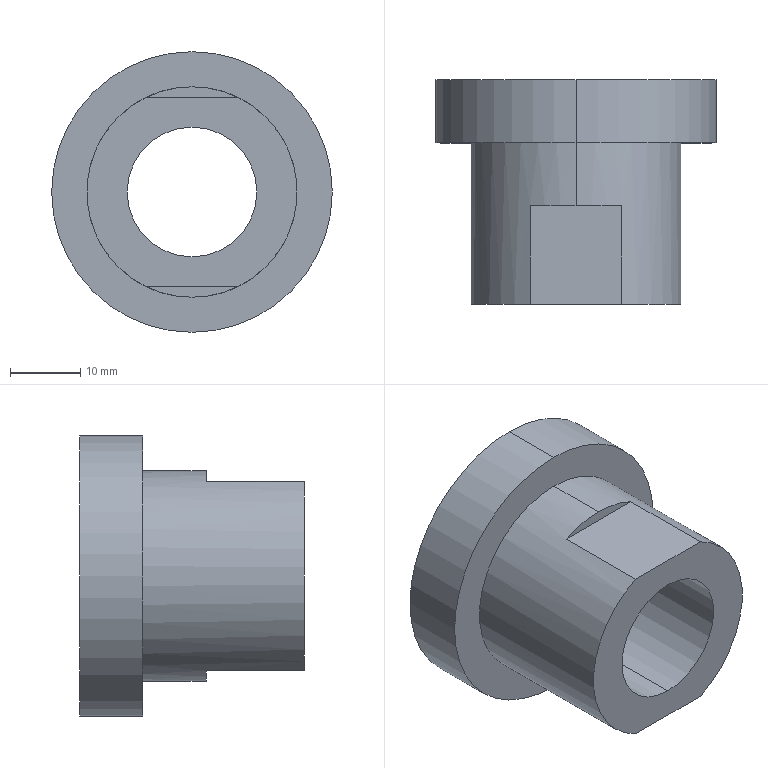Part | SolidWorks | features ICE 2, Extrusion 1, HoleWzd 1 | 1 solid | 13 faces | box 40 x 32 x 40 mm | volume 18596 mm3 | plane 7 | cylinder 6 | commonest cylinder face diameters 18.5 x2 30 x2 40 x2
STEP:
#1=CARTESIAN_POINT('',(0.,0.,-9.25));
#2=VERTEX_POINT('',#1);
#3=CARTESIAN_POINT('',(0.,0.,9.25));
#4=VERTEX_POINT('',#3);
#5=CARTESIAN_POINT('',(0.,0.,0.));
#6=DIRECTION('',(0.,1.,0.));
#7=DIRECTION('',(0.,0.,1.));
#8=AXIS2_PLACEMENT_3D('',#5,#6,#7);
#9=CIRCLE('',#8,9.25);
#10=EDGE_CURVE('',#2,#4,#9,.T.);
#11=ORIENTED_EDGE('',*,*,#10,.F.);
#12=CARTESIAN_POINT('',(0.,32.,-9.25));
#13=VERTEX_POINT('',#12);
#14=CARTESIAN_POINT('',(0.,32.,-9.25));
#15=DIRECTION('',(0.,1.,0.));
#16=VECTOR('',#15,1000.);
#17=LINE('',#14,#16);
#18=EDGE_CURVE('',#2,#13,#17,.T.);
#19=ORIENTED_EDGE('',*,*,#18,.T.);
#20=CARTESIAN_POINT('',(0.,32.,9.25));
#21=VERTEX_POINT('',#20);
#22=CARTESIAN_POINT('',(0.,32.,0.));
#23=DIRECTION('',(0.,1.,0.));
#24=DIRECTION('',(0.,0.,1.));
#25=AXIS2_PLACEMENT_3D('',#22,#23,#24);
#26=CIRCLE('',#25,9.25);
#27=EDGE_CURVE('',#13,#21,#26,.T.);
#28=ORIENTED_EDGE('',*,*,#27,.T.);
#29=CARTESIAN_POINT('',(0.,32.,9.25));
#30=DIRECTION('',(0.,1.,0.));
#31=VECTOR('',#30,1000.);
#32=LINE('',#29,#31);
#33=EDGE_CURVE('',#4,#21,#32,.T.);
#34=ORIENTED_EDGE('',*,*,#33,.F.);
#35=EDGE_LOOP('',(#11,#19,#28,#34));
#36=FACE_OUTER_BOUND('',#35,.T.);
#37=CARTESIAN_POINT('',(0.,32.,0.));
#38=DIRECTION('',(0.,1.,0.));
#39=DIRECTION('',(0.,0.,1.));
#40=AXIS2_PLACEMENT_3D('',#37,#38,#39);
#41=CYLINDRICAL_SURFACE('',#40,9.25);
#42=ADVANCED_FACE('',(#36),#41,.F.);
#43=CARTESIAN_POINT('',(0.,23.,-15.));
#44=VERTEX_POINT('',#43);
#45=CARTESIAN_POINT('',(0.,23.,15.));
#46=VERTEX_POINT('',#45);
#47=CARTESIAN_POINT('',(0.,23.,0.));
#48=DIRECTION('',(0.,-1.,0.));
#49=DIRECTION('',(0.,0.,-1.));
#50=AXIS2_PLACEMENT_3D('',#47,#48,#49);
#51=CIRCLE('',#50,15.);
#52=EDGE_CURVE('',#44,#46,#51,.T.);
#53=ORIENTED_EDGE('',*,*,#52,.T.);
#54=CARTESIAN_POINT('',(0.,14.,15.));
#55=VERTEX_POINT('',#54);
#56=CARTESIAN_POINT('',(0.,23.,15.));
#57=DIRECTION('',(0.,-1.,0.));
#58=VECTOR('',#57,1000.);
#59=LINE('',#56,#58);
#60=EDGE_CURVE('',#46,#55,#59,.T.);
#61=ORIENTED_EDGE('',*,*,#60,.T.);
#62=CARTESIAN_POINT('',(6.538,14.,13.5));
#63=VERTEX_POINT('',#62);
#64=CARTESIAN_POINT('',(0.,14.,0.));
#65=DIRECTION('',(0.,-1.,0.));
#66=DIRECTION('',(0.,0.,1.));
#67=AXIS2_PLACEMENT_3D('',#64,#65,#66);
#68=CIRCLE('',#67,15.);
#69=EDGE_CURVE('',#63,#55,#68,.T.);
#70=ORIENTED_EDGE('',*,*,#69,.F.);
#71=CARTESIAN_POINT('',(6.538,0.,13.5));
#72=VERTEX_POINT('',#71);
#73=CARTESIAN_POINT('',(6.538,23.,13.5));
#74=DIRECTION('',(0.,1.,0.));
#75=VECTOR('',#74,1000.);
#76=LINE('',#73,#75);
#77=EDGE_CURVE('',#72,#63,#76,.T.);
#78=ORIENTED_EDGE('',*,*,#77,.F.);
#79=CARTESIAN_POINT('',(6.538,0.,-13.5));
#80=VERTEX_POINT('',#79);
#81=CARTESIAN_POINT('',(0.,0.,0.));
#82=DIRECTION('',(0.,-1.,0.));
#83=DIRECTION('',(0.,0.,-1.));
#84=AXIS2_PLACEMENT_3D('',#81,#82,#83);
#85=CIRCLE('',#84,15.);
#86=EDGE_CURVE('',#80,#72,#85,.T.);
#87=ORIENTED_EDGE('',*,*,#86,.F.);
#88=CARTESIAN_POINT('',(6.538,14.,-13.5));
#89=VERTEX_POINT('',#88);
#90=CARTESIAN_POINT('',(6.538,23.,-13.5));
#91=DIRECTION('',(0.,-1.,0.));
#92=VECTOR('',#91,1000.);
#93=LINE('',#90,#92);
#94=EDGE_CURVE('',#89,#80,#93,.T.);
#95=ORIENTED_EDGE('',*,*,#94,.F.);
#96=CARTESIAN_POINT('',(0.,14.,-15.));
#97=VERTEX_POINT('',#96);
#98=CARTESIAN_POINT('',(0.,14.,0.));
#99=DIRECTION('',(0.,-1.,0.));
#100=DIRECTION('',(0.,0.,1.));
#101=AXIS2_PLACEMENT_3D('',#98,#99,#100);
#102=CIRCLE('',#101,15.);
#103=EDGE_CURVE('',#97,#89,#102,.T.);
#104=ORIENTED_EDGE('',*,*,#103,.F.);
#105=CARTESIAN_POINT('',(0.,23.,-15.));
#106=DIRECTION('',(0.,-1.,0.));
#107=VECTOR('',#106,1000.);
#108=LINE('',#105,#107);
#109=EDGE_CURVE('',#44,#97,#108,.T.);
#110=ORIENTED_EDGE('',*,*,#109,.F.);
#111=EDGE_LOOP('',(#53,#61,#70,#78,#87,#95,#104,#110));
#112=FACE_OUTER_BOUND('',#111,.T.);
#113=CARTESIAN_POINT('',(0.,23.,0.));
#114=DIRECTION('',(0.,-1.,0.));
#115=DIRECTION('',(0.,0.,-1.));
#116=AXIS2_PLACEMENT_3D('',#113,#114,#115);
#117=CYLINDRICAL_SURFACE('',#116,15.);
#118=ADVANCED_FACE('',(#112),#117,.T.);
#119=CARTESIAN_POINT('',(0.,32.,20.));
#120=VERTEX_POINT('',#119);
#121=CARTESIAN_POINT('',(0.,32.,-20.));
#122=VERTEX_POINT('',#121);
#123=CARTESIAN_POINT('',(0.,32.,0.));
#124=DIRECTION('',(0.,1.,0.));
#125=DIRECTION('',(0.,0.,1.));
#126=AXIS2_PLACEMENT_3D('',#123,#124,#125);
#127=CIRCLE('',#126,20.);
#128=EDGE_CURVE('',#120,#122,#127,.T.);
#129=ORIENTED_EDGE('',*,*,#128,.F.);
#130=CARTESIAN_POINT('',(0.,23.,20.));
#131=VERTEX_POINT('',#130);
#132=CARTESIAN_POINT('',(0.,32.,20.));
#133=DIRECTION('',(0.,-1.,0.));
#134=VECTOR('',#133,1000.);
#135=LINE('',#132,#134);
#136=EDGE_CURVE('',#120,#131,#135,.T.);
#137=ORIENTED_EDGE('',*,*,#136,.T.);
#138=CARTESIAN_POINT('',(0.,23.,-20.));
#139=VERTEX_POINT('',#138);
#140=CARTESIAN_POINT('',(0.,23.,0.));
#141=DIRECTION('',(0.,-1.,0.));
#142=DIRECTION('',(0.,0.,-1.));
#143=AXIS2_PLACEMENT_3D('',#140,#141,#142);
#144=CIRCLE('',#143,20.);
#145=EDGE_CURVE('',#139,#131,#144,.T.);
#146=ORIENTED_EDGE('',*,*,#145,.F.);
#147=CARTESIAN_POINT('',(0.,32.,-20.));
#148=DIRECTION('',(0.,-1.,0.));
#149=VECTOR('',#148,1000.);
#150=LINE('',#147,#149);
#151=EDGE_CURVE('',#122,#139,#150,.T.);
#152=ORIENTED_EDGE('',*,*,#151,.F.);
#153=EDGE_LOOP('',(#129,#137,#146,#152));
#154=FACE_OUTER_BOUND('',#153,.T.);
#155=CARTESIAN_POINT('',(0.,32.,0.));
#156=DIRECTION('',(0.,-1.,0.));
#157=DIRECTION('',(0.,0.,-1.));
#158=AXIS2_PLACEMENT_3D('',#155,#156,#157);
#159=CYLINDRICAL_SURFACE('',#158,20.);
#160=ADVANCED_FACE('',(#154),#159,.T.);
#161=CARTESIAN_POINT('',(0.,0.,0.));
#162=DIRECTION('',(0.,1.,0.));
#163=DIRECTION('',(0.,0.,1.));
#164=AXIS2_PLACEMENT_3D('',#161,#162,#163);
#165=CIRCLE('',#164,9.25);
#166=EDGE_CURVE('',#4,#2,#165,.T.);
#167=ORIENTED_EDGE('',*,*,#166,.T.);
#168=ORIENTED_EDGE('',*,*,#10,.T.);
#169=EDGE_LOOP('',(#167,#168));
#170=FACE_BOUND('',#169,.T.);
#171=ORIENTED_EDGE('',*,*,#86,.T.);
#172=CARTESIAN_POINT('',(-6.538,0.,13.5));
#173=VERTEX_POINT('',#172);
#174=CARTESIAN_POINT('',(0.,0.,13.5));
#175=DIRECTION('',(-1.,0.,0.));
#176=VECTOR('',#175,1000.);
#177=LINE('',#174,#176);
#178=EDGE_CURVE('',#72,#173,#177,.T.);
#179=ORIENTED_EDGE('',*,*,#178,.T.);
#180=CARTESIAN_POINT('',(-6.538,0.,-13.5));
#181=VERTEX_POINT('',#180);
#182=CARTESIAN_POINT('',(0.,0.,0.));
#183=DIRECTION('',(0.,-1.,0.));
#184=DIRECTION('',(0.,0.,-1.));
#185=AXIS2_PLACEMENT_3D('',#182,#183,#184);
#186=CIRCLE('',#185,15.);
#187=EDGE_CURVE('',#173,#181,#186,.T.);
#188=ORIENTED_EDGE('',*,*,#187,.T.);
#189=CARTESIAN_POINT('',(0.,0.,-13.5));
#190=DIRECTION('',(1.,0.,0.));
#191=VECTOR('',#190,1000.);
#192=LINE('',#189,#191);
#193=EDGE_CURVE('',#181,#80,#192,.T.);
#194=ORIENTED_EDGE('',*,*,#193,.T.);
#195=EDGE_LOOP('',(#171,#179,#188,#194));
#196=FACE_OUTER_BOUND('',#195,.T.);
#197=CARTESIAN_POINT('',(0.,0.,0.));
#198=DIRECTION('',(0.,1.,0.));
#199=DIRECTION('',(0.,0.,1.));
#200=AXIS2_PLACEMENT_3D('',#197,#198,#199);
#201=PLANE('',#200);
#202=ADVANCED_FACE('',(#170,#196),#201,.F.);
#203=ORIENTED_EDGE('',*,*,#136,.F.);
#204=CARTESIAN_POINT('',(0.,32.,0.));
#205=DIRECTION('',(0.,1.,0.));
#206=DIRECTION('',(0.,0.,1.));
#207=AXIS2_PLACEMENT_3D('',#204,#205,#206);
#208=CIRCLE('',#207,20.);
#209=EDGE_CURVE('',#122,#120,#208,.T.);
#210=ORIENTED_EDGE('',*,*,#209,.F.);
#211=ORIENTED_EDGE('',*,*,#151,.T.);
#212=CARTESIAN_POINT('',(0.,23.,0.));
#213=DIRECTION('',(0.,-1.,0.));
#214=DIRECTION('',(0.,0.,-1.));
#215=AXIS2_PLACEMENT_3D('',#212,#213,#214);
#216=CIRCLE('',#215,20.);
#217=EDGE_CURVE('',#131,#139,#216,.T.);
#218=ORIENTED_EDGE('',*,*,#217,.F.);
#219=EDGE_LOOP('',(#203,#210,#211,#218));
#220=FACE_OUTER_BOUND('',#219,.T.);
#221=CARTESIAN_POINT('',(0.,32.,0.));
#222=DIRECTION('',(0.,-1.,0.));
#223=DIRECTION('',(0.,0.,-1.));
#224=AXIS2_PLACEMENT_3D('',#221,#222,#223);
#225=CYLINDRICAL_SURFACE('',#224,20.);
#226=ADVANCED_FACE('',(#220),#225,.T.);
#227=CARTESIAN_POINT('',(0.,32.,0.));
#228=DIRECTION('',(0.,1.,0.));
#229=DIRECTION('',(0.,0.,1.));
#230=AXIS2_PLACEMENT_3D('',#227,#228,#229);
#231=CIRCLE('',#230,9.25);
#232=EDGE_CURVE('',#21,#13,#231,.T.);
#233=ORIENTED_EDGE('',*,*,#232,.F.);
#234=ORIENTED_EDGE('',*,*,#27,.F.);
#235=EDGE_LOOP('',(#233,#234));
#236=FACE_BOUND('',#235,.T.);
#237=ORIENTED_EDGE('',*,*,#209,.T.);
#238=ORIENTED_EDGE('',*,*,#128,.T.);
#239=EDGE_LOOP('',(#237,#238));
#240=FACE_OUTER_BOUND('',#239,.T.);
#241=CARTESIAN_POINT('',(0.,32.,0.));
#242=DIRECTION('',(0.,1.,0.));
#243=DIRECTION('',(0.,0.,1.));
#244=AXIS2_PLACEMENT_3D('',#241,#242,#243);
#245=PLANE('',#244);
#246=ADVANCED_FACE('',(#236,#240),#245,.T.);
#247=ORIENTED_EDGE('',*,*,#52,.F.);
#248=CARTESIAN_POINT('',(0.,23.,0.));
#249=DIRECTION('',(0.,-1.,0.));
#250=DIRECTION('',(0.,0.,-1.));
#251=AXIS2_PLACEMENT_3D('',#248,#249,#250);
#252=CIRCLE('',#251,15.);
#253=EDGE_CURVE('',#46,#44,#252,.T.);
#254=ORIENTED_EDGE('',*,*,#253,.F.);
#255=EDGE_LOOP('',(#247,#254));
#256=FACE_BOUND('',#255,.T.);
#257=ORIENTED_EDGE('',*,*,#145,.T.);
#258=ORIENTED_EDGE('',*,*,#217,.T.);
#259=EDGE_LOOP('',(#257,#258));
#260=FACE_OUTER_BOUND('',#259,.T.);
#261=CARTESIAN_POINT('',(0.,23.,0.));
#262=DIRECTION('',(0.,-1.,0.));
#263=DIRECTION('',(0.,0.,-1.));
#264=AXIS2_PLACEMENT_3D('',#261,#262,#263);
#265=PLANE('',#264);
#266=ADVANCED_FACE('',(#256,#260),#265,.T.);
#267=ORIENTED_EDGE('',*,*,#60,.F.);
#268=ORIENTED_EDGE('',*,*,#253,.T.);
#269=ORIENTED_EDGE('',*,*,#109,.T.);
#270=CARTESIAN_POINT('',(-6.538,14.,-13.5));
#271=VERTEX_POINT('',#270);
#272=CARTESIAN_POINT('',(0.,14.,0.));
#273=DIRECTION('',(0.,-1.,0.));
#274=DIRECTION('',(0.,0.,1.));
#275=AXIS2_PLACEMENT_3D('',#272,#273,#274);
#276=CIRCLE('',#275,15.);
#277=EDGE_CURVE('',#271,#97,#276,.T.);
#278=ORIENTED_EDGE('',*,*,#277,.F.);
#279=CARTESIAN_POINT('',(-6.538,23.,-13.5));
#280=DIRECTION('',(0.,1.,0.));
#281=VECTOR('',#280,1000.);
#282=LINE('',#279,#281);
#283=EDGE_CURVE('',#181,#271,#282,.T.);
#284=ORIENTED_EDGE('',*,*,#283,.F.);
#285=ORIENTED_EDGE('',*,*,#187,.F.);
#286=CARTESIAN_POINT('',(-6.538,14.,13.5));
#287=VERTEX_POINT('',#286);
#288=CARTESIAN_POINT('',(-6.538,23.,13.5));
#289=DIRECTION('',(0.,-1.,0.));
#290=VECTOR('',#289,1000.);
#291=LINE('',#288,#290);
#292=EDGE_CURVE('',#287,#173,#291,.T.);
#293=ORIENTED_EDGE('',*,*,#292,.F.);
#294=CARTESIAN_POINT('',(0.,14.,0.));
#295=DIRECTION('',(0.,-1.,0.));
#296=DIRECTION('',(0.,0.,1.));
#297=AXIS2_PLACEMENT_3D('',#294,#295,#296);
#298=CIRCLE('',#297,15.);
#299=EDGE_CURVE('',#55,#287,#298,.T.);
#300=ORIENTED_EDGE('',*,*,#299,.F.);
#301=EDGE_LOOP('',(#267,#268,#269,#278,#284,#285,#293,#300));
#302=FACE_OUTER_BOUND('',#301,.T.);
#303=CARTESIAN_POINT('',(0.,23.,0.));
#304=DIRECTION('',(0.,-1.,0.));
#305=DIRECTION('',(0.,0.,-1.));
#306=AXIS2_PLACEMENT_3D('',#303,#304,#305);
#307=CYLINDRICAL_SURFACE('',#306,15.);
#308=ADVANCED_FACE('',(#302),#307,.T.);
#309=ORIENTED_EDGE('',*,*,#277,.T.);
#310=ORIENTED_EDGE('',*,*,#103,.T.);
#311=CARTESIAN_POINT('',(-20.,14.,-13.5));
#312=DIRECTION('',(1.,0.,0.));
#313=VECTOR('',#312,1000.);
#314=LINE('',#311,#313);
#315=EDGE_CURVE('',#271,#89,#314,.T.);
#316=ORIENTED_EDGE('',*,*,#315,.F.);
#317=EDGE_LOOP('',(#309,#310,#316));
#318=FACE_OUTER_BOUND('',#317,.T.);
#319=CARTESIAN_POINT('',(-20.,14.,-20.989));
#320=DIRECTION('',(0.,1.,0.));
#321=DIRECTION('',(0.,0.,1.));
#322=AXIS2_PLACEMENT_3D('',#319,#320,#321);
#323=PLANE('',#322);
#324=ADVANCED_FACE('',(#318),#323,.F.);
#325=ORIENTED_EDGE('',*,*,#283,.T.);
#326=ORIENTED_EDGE('',*,*,#315,.T.);
#327=ORIENTED_EDGE('',*,*,#94,.T.);
#328=ORIENTED_EDGE('',*,*,#193,.F.);
#329=EDGE_LOOP('',(#325,#326,#327,#328));
#330=FACE_OUTER_BOUND('',#329,.T.);
#331=CARTESIAN_POINT('',(-20.,14.,-13.5));
#332=DIRECTION('',(0.,0.,1.));
#333=DIRECTION('',(0.,-1.,0.));
#334=AXIS2_PLACEMENT_3D('',#331,#332,#333);
#335=PLANE('',#334);
#336=ADVANCED_FACE('',(#330),#335,.F.);
#337=ORIENTED_EDGE('',*,*,#69,.T.);
#338=ORIENTED_EDGE('',*,*,#299,.T.);
#339=CARTESIAN_POINT('',(-20.,14.,13.5));
#340=DIRECTION('',(1.,0.,0.));
#341=VECTOR('',#340,1000.);
#342=LINE('',#339,#341);
#343=EDGE_CURVE('',#287,#63,#342,.T.);
#344=ORIENTED_EDGE('',*,*,#343,.T.);
#345=EDGE_LOOP('',(#337,#338,#344));
#346=FACE_OUTER_BOUND('',#345,.T.);
#347=CARTESIAN_POINT('',(-20.,14.,20.989));
#348=DIRECTION('',(0.,1.,0.));
#349=DIRECTION('',(0.,0.,1.));
#350=AXIS2_PLACEMENT_3D('',#347,#348,#349);
#351=PLANE('',#350);
#352=ADVANCED_FACE('',(#346),#351,.F.);
#353=ORIENTED_EDGE('',*,*,#77,.T.);
#354=ORIENTED_EDGE('',*,*,#343,.F.);
#355=ORIENTED_EDGE('',*,*,#292,.T.);
#356=ORIENTED_EDGE('',*,*,#178,.F.);
#357=EDGE_LOOP('',(#353,#354,#355,#356));
#358=FACE_OUTER_BOUND('',#357,.T.);
#359=CARTESIAN_POINT('',(-20.,14.,13.5));
#360=DIRECTION('',(0.,0.,-1.));
#361=DIRECTION('',(0.,1.,0.));
#362=AXIS2_PLACEMENT_3D('',#359,#360,#361);
#363=PLANE('',#362);
#364=ADVANCED_FACE('',(#358),#363,.F.);
#365=ORIENTED_EDGE('',*,*,#18,.F.);
#366=ORIENTED_EDGE('',*,*,#166,.F.);
#367=ORIENTED_EDGE('',*,*,#33,.T.);
#368=ORIENTED_EDGE('',*,*,#232,.T.);
#369=EDGE_LOOP('',(#365,#366,#367,#368));
#370=FACE_OUTER_BOUND('',#369,.T.);
#371=CARTESIAN_POINT('',(0.,32.,0.));
#372=DIRECTION('',(0.,1.,0.));
#373=DIRECTION('',(0.,0.,1.));
#374=AXIS2_PLACEMENT_3D('',#371,#372,#373);
#375=CYLINDRICAL_SURFACE('',#374,9.25);
#376=ADVANCED_FACE('',(#370),#375,.F.);
#377=CLOSED_SHELL('',(#42,#118,#160,#202,#226,#246,#266,#308,#324,#336,#352,#364,#376));
#378=MANIFOLD_SOLID_BREP('',#377);
#379=CARTESIAN_POINT('',(0.,0.,0.));
#380=DIRECTION('',(0.,0.,1.));
#381=DIRECTION('',(1.,0.,0.));
#382=AXIS2_PLACEMENT_3D('',#379,#380,#381);
#383=(LENGTH_UNIT()NAMED_UNIT(*)SI_UNIT(.MILLI.,.METRE.));
#384=UNCERTAINTY_MEASURE_WITH_UNIT(LENGTH_MEASURE(0.00001),#383,'','');
#385=(NAMED_UNIT(*)PLANE_ANGLE_UNIT()SI_UNIT($,.RADIAN.));
#386=(NAMED_UNIT(*)SI_UNIT($,.STERADIAN.)SOLID_ANGLE_UNIT());
#387=(GEOMETRIC_REPRESENTATION_CONTEXT(3)GLOBAL_UNCERTAINTY_ASSIGNED_CONTEXT((#384))GLOBAL_UNIT_ASSIGNED_CONTEXT((#383,#385,#386))REPRESENTATION_CONTEXT('',''));
#388=ADVANCED_BREP_SHAPE_REPRESENTATION('',(#378,#382),#387);